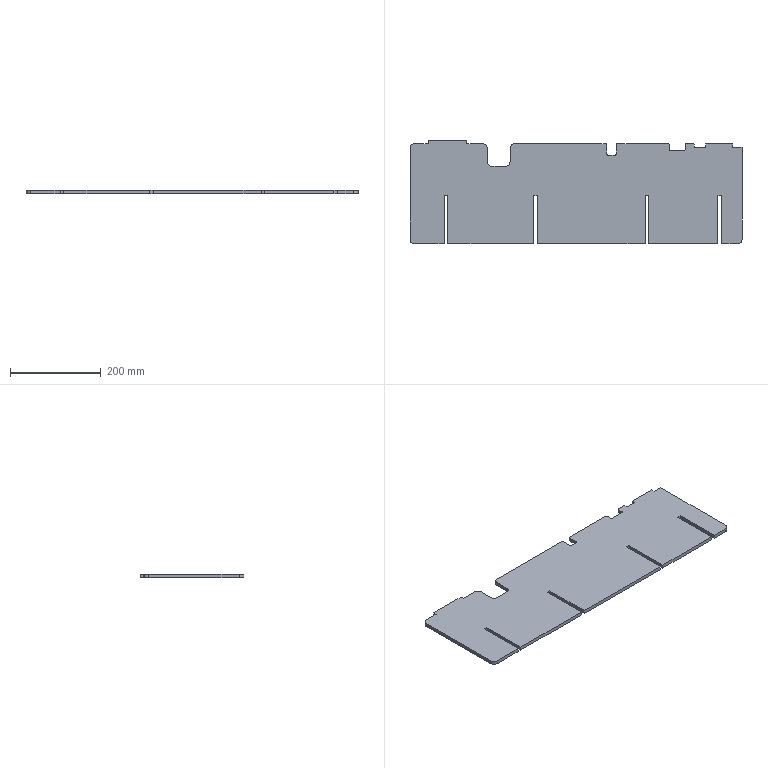Part | SolidWorks | features FlatPattern 1, SMBaseFlange 1, SheetMetal 1 | 1 solid | 61 faces | box 730 x 227.5 x 8 mm | volume 1230929 mm3 | plane 44 | cylinder 17 | commonest cylinder face diameters 4 x10 20 x7